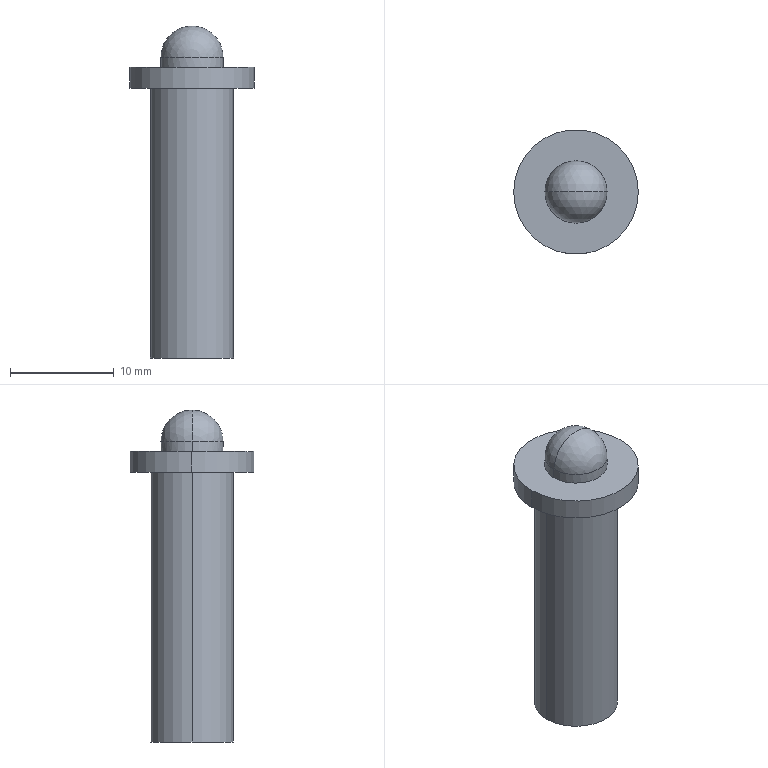Part | STEP file | 2053 Spring mounting seat A | 1 solid | 15 faces | box 12 x 12 x 32 mm | volume 1418 mm3 | cylinder 8 | plane 3 | cone 2 | sphere 2 | commonest cylinder face diameters 4.2 x2 6 x2 8 x2 12 x2
STEP:
#1=CARTESIAN_POINT('',(0.,0.,0.));
#2=DIRECTION('',(0.,0.,1.));
#3=DIRECTION('',(1.,0.,0.));
#4=AXIS2_PLACEMENT_3D('',#1,#2,#3);
#5=CARTESIAN_POINT('',(-2.1,0.,-14.));
#6=VERTEX_POINT('',#5);
#7=CARTESIAN_POINT('',(-2.1,0.,-28.));
#8=VERTEX_POINT('',#7);
#9=CARTESIAN_POINT('',(-2.1,0.,-28.));
#10=DIRECTION('',(0.,0.,-1.));
#11=VECTOR('',#10,1.);
#12=LINE('',#9,#11);
#13=CARTESIAN_POINT('',(0.,0.,-28.));
#14=DIRECTION('',(0.,0.,-1.));
#15=DIRECTION('',(-1.,0.,0.));
#16=AXIS2_PLACEMENT_3D('',#13,#14,#15);
#17=CYLINDRICAL_SURFACE('',#16,2.1);
#18=CARTESIAN_POINT('',(6.283,0.));
#19=DIRECTION('',(0.,1.));
#20=VECTOR('',#19,1.);
#21=LINE('',#18,#20);
#22=(GEOMETRIC_REPRESENTATION_CONTEXT(2)PARAMETRIC_REPRESENTATION_CONTEXT()REPRESENTATION_CONTEXT('',''));
#23=DEFINITIONAL_REPRESENTATION('',(#21),#22);
#24=PCURVE('',#17,#23);
#25=CARTESIAN_POINT('',(0.,0.,-28.));
#26=DIRECTION('',(0.,0.,-1.));
#27=DIRECTION('',(-1.,0.,0.));
#28=AXIS2_PLACEMENT_3D('',#25,#26,#27);
#29=CYLINDRICAL_SURFACE('',#28,2.1);
#30=CARTESIAN_POINT('',(0.,0.));
#31=DIRECTION('',(0.,1.));
#32=VECTOR('',#31,1.);
#33=LINE('',#30,#32);
#34=(GEOMETRIC_REPRESENTATION_CONTEXT(2)PARAMETRIC_REPRESENTATION_CONTEXT()REPRESENTATION_CONTEXT('',''));
#35=DEFINITIONAL_REPRESENTATION('',(#33),#34);
#36=PCURVE('',#29,#35);
#37=SURFACE_CURVE('',#12,(#24,#36),.PCURVE_S1.);
#38=EDGE_CURVE('',#6,#8,#37,.T.);
#39=ORIENTED_EDGE('',*,*,#38,.T.);
#40=CARTESIAN_POINT('',(2.1,0.,-28.));
#41=VERTEX_POINT('',#40);
#42=CARTESIAN_POINT('',(0.,0.,-28.));
#43=DIRECTION('',(0.,0.,-1.));
#44=DIRECTION('',(-1.,0.,0.));
#45=AXIS2_PLACEMENT_3D('',#42,#43,#44);
#46=CIRCLE('',#45,2.1);
#47=CARTESIAN_POINT('',(0.,0.));
#48=DIRECTION('',(1.,0.));
#49=VECTOR('',#48,1.);
#50=LINE('',#47,#49);
#51=(GEOMETRIC_REPRESENTATION_CONTEXT(2)PARAMETRIC_REPRESENTATION_CONTEXT()REPRESENTATION_CONTEXT('',''));
#52=DEFINITIONAL_REPRESENTATION('',(#50),#51);
#53=PCURVE('',#17,#52);
#54=CARTESIAN_POINT('',(0.,0.,-28.));
#55=DIRECTION('',(0.,0.,-1.));
#56=DIRECTION('',(-1.,0.,0.));
#57=AXIS2_PLACEMENT_3D('',#54,#55,#56);
#58=PLANE('',#57);
#59=CARTESIAN_POINT('',(0.,0.));
#60=DIRECTION('',(1.,0.));
#61=AXIS2_PLACEMENT_2D('',#59,#60);
#62=CIRCLE('',#61,2.1);
#63=(GEOMETRIC_REPRESENTATION_CONTEXT(2)PARAMETRIC_REPRESENTATION_CONTEXT()REPRESENTATION_CONTEXT('',''));
#64=DEFINITIONAL_REPRESENTATION('',(#62),#63);
#65=PCURVE('',#58,#64);
#66=SURFACE_CURVE('',#46,(#53,#65),.PCURVE_S1.);
#67=EDGE_CURVE('',#41,#8,#66,.T.);
#68=ORIENTED_EDGE('',*,*,#67,.F.);
#69=CARTESIAN_POINT('',(2.1,0.,-14.));
#70=VERTEX_POINT('',#69);
#71=CARTESIAN_POINT('',(2.1,0.,-28.));
#72=DIRECTION('',(0.,0.,-1.));
#73=VECTOR('',#72,1.);
#74=LINE('',#71,#73);
#75=CARTESIAN_POINT('',(3.142,0.));
#76=DIRECTION('',(0.,1.));
#77=VECTOR('',#76,1.);
#78=LINE('',#75,#77);
#79=(GEOMETRIC_REPRESENTATION_CONTEXT(2)PARAMETRIC_REPRESENTATION_CONTEXT()REPRESENTATION_CONTEXT('',''));
#80=DEFINITIONAL_REPRESENTATION('',(#78),#79);
#81=PCURVE('',#17,#80);
#82=CARTESIAN_POINT('',(3.142,0.));
#83=DIRECTION('',(0.,1.));
#84=VECTOR('',#83,1.);
#85=LINE('',#82,#84);
#86=(GEOMETRIC_REPRESENTATION_CONTEXT(2)PARAMETRIC_REPRESENTATION_CONTEXT()REPRESENTATION_CONTEXT('',''));
#87=DEFINITIONAL_REPRESENTATION('',(#85),#86);
#88=PCURVE('',#29,#87);
#89=SURFACE_CURVE('',#74,(#81,#88),.PCURVE_S1.);
#90=EDGE_CURVE('',#70,#41,#89,.T.);
#91=ORIENTED_EDGE('',*,*,#90,.F.);
#92=CARTESIAN_POINT('',(0.,0.,-14.));
#93=DIRECTION('',(0.,0.,-1.));
#94=DIRECTION('',(-1.,0.,0.));
#95=AXIS2_PLACEMENT_3D('',#92,#93,#94);
#96=CIRCLE('',#95,2.1);
#97=CARTESIAN_POINT('',(0.,-14.));
#98=DIRECTION('',(1.,0.));
#99=VECTOR('',#98,1.);
#100=LINE('',#97,#99);
#101=(GEOMETRIC_REPRESENTATION_CONTEXT(2)PARAMETRIC_REPRESENTATION_CONTEXT()REPRESENTATION_CONTEXT('',''));
#102=DEFINITIONAL_REPRESENTATION('',(#100),#101);
#103=PCURVE('',#17,#102);
#104=CARTESIAN_POINT('',(0.,0.,-14.));
#105=DIRECTION('',(0.,0.,-1.));
#106=DIRECTION('',(-1.,0.,0.));
#107=AXIS2_PLACEMENT_3D('',#104,#105,#106);
#108=CONICAL_SURFACE('',#107,2.1,1.03);
#109=CARTESIAN_POINT('',(0.,0.));
#110=DIRECTION('',(1.,0.));
#111=VECTOR('',#110,1.);
#112=LINE('',#109,#111);
#113=(GEOMETRIC_REPRESENTATION_CONTEXT(2)PARAMETRIC_REPRESENTATION_CONTEXT()REPRESENTATION_CONTEXT('',''));
#114=DEFINITIONAL_REPRESENTATION('',(#112),#113);
#115=PCURVE('',#108,#114);
#116=SURFACE_CURVE('',#96,(#103,#115),.PCURVE_S1.);
#117=EDGE_CURVE('',#70,#6,#116,.T.);
#118=ORIENTED_EDGE('',*,*,#117,.T.);
#119=EDGE_LOOP('',(#39,#68,#91,#118));
#120=FACE_BOUND('',#119,.F.);
#121=ADVANCED_FACE('',(#120),#17,.F.);
#122=ORIENTED_EDGE('',*,*,#117,.F.);
#123=CARTESIAN_POINT('',(0.,0.,-12.738));
#124=VERTEX_POINT('',#123);
#125=CARTESIAN_POINT('',(2.1,0.,-14.));
#126=DIRECTION('',(0.8572,0.,-0.515));
#127=VECTOR('',#126,1.);
#128=LINE('',#125,#127);
#129=CARTESIAN_POINT('',(3.142,0.));
#130=DIRECTION('',(0.,1.));
#131=VECTOR('',#130,1.);
#132=LINE('',#129,#131);
#133=(GEOMETRIC_REPRESENTATION_CONTEXT(2)PARAMETRIC_REPRESENTATION_CONTEXT()REPRESENTATION_CONTEXT('',''));
#134=DEFINITIONAL_REPRESENTATION('',(#132),#133);
#135=PCURVE('',#108,#134);
#136=CARTESIAN_POINT('',(0.,0.,-14.));
#137=DIRECTION('',(0.,0.,-1.));
#138=DIRECTION('',(-1.,0.,0.));
#139=AXIS2_PLACEMENT_3D('',#136,#137,#138);
#140=CONICAL_SURFACE('',#139,2.1,1.03);
#141=CARTESIAN_POINT('',(3.142,0.));
#142=DIRECTION('',(0.,1.));
#143=VECTOR('',#142,1.);
#144=LINE('',#141,#143);
#145=(GEOMETRIC_REPRESENTATION_CONTEXT(2)PARAMETRIC_REPRESENTATION_CONTEXT()REPRESENTATION_CONTEXT('',''));
#146=DEFINITIONAL_REPRESENTATION('',(#144),#145);
#147=PCURVE('',#140,#146);
#148=SURFACE_CURVE('',#128,(#135,#147),.PCURVE_S1.);
#149=EDGE_CURVE('',#124,#70,#148,.T.);
#150=ORIENTED_EDGE('',*,*,#149,.F.);
#151=CARTESIAN_POINT('',(-2.1,0.,-14.));
#152=DIRECTION('',(-0.8572,0.,-0.515));
#153=VECTOR('',#152,1.);
#154=LINE('',#151,#153);
#155=CARTESIAN_POINT('',(6.283,0.));
#156=DIRECTION('',(0.,1.));
#157=VECTOR('',#156,1.);
#158=LINE('',#155,#157);
#159=(GEOMETRIC_REPRESENTATION_CONTEXT(2)PARAMETRIC_REPRESENTATION_CONTEXT()REPRESENTATION_CONTEXT('',''));
#160=DEFINITIONAL_REPRESENTATION('',(#158),#159);
#161=PCURVE('',#108,#160);
#162=CARTESIAN_POINT('',(0.,0.));
#163=DIRECTION('',(0.,1.));
#164=VECTOR('',#163,1.);
#165=LINE('',#162,#164);
#166=(GEOMETRIC_REPRESENTATION_CONTEXT(2)PARAMETRIC_REPRESENTATION_CONTEXT()REPRESENTATION_CONTEXT('',''));
#167=DEFINITIONAL_REPRESENTATION('',(#165),#166);
#168=PCURVE('',#140,#167);
#169=SURFACE_CURVE('',#154,(#161,#168),.PCURVE_S1.);
#170=EDGE_CURVE('',#124,#6,#169,.T.);
#171=ORIENTED_EDGE('',*,*,#170,.T.);
#172=EDGE_LOOP('',(#122,#150,#171));
#173=FACE_BOUND('',#172,.F.);
#174=ADVANCED_FACE('',(#173),#108,.F.);
#175=CARTESIAN_POINT('',(0.,3.,1.));
#176=VERTEX_POINT('',#175);
#177=CARTESIAN_POINT('',(3.,0.,1.));
#178=VERTEX_POINT('',#177);
#179=CARTESIAN_POINT('',(0.,0.,1.));
#180=DIRECTION('',(0.,0.,-1.));
#181=DIRECTION('',(-1.,0.,0.));
#182=AXIS2_PLACEMENT_3D('',#179,#180,#181);
#183=CIRCLE('',#182,3.);
#184=CARTESIAN_POINT('',(0.,0.,1.));
#185=DIRECTION('',(0.,1.,0.));
#186=DIRECTION('',(1.,0.,0.));
#187=AXIS2_PLACEMENT_3D('',#184,#185,#186);
#188=SPHERICAL_SURFACE('',#187,3.);
#189=CARTESIAN_POINT('',(6.283,1.571));
#190=CARTESIAN_POINT('',(6.283,1.547));
#191=CARTESIAN_POINT('',(6.283,1.499));
#192=CARTESIAN_POINT('',(6.283,1.428));
#193=CARTESIAN_POINT('',(6.283,1.357));
#194=CARTESIAN_POINT('',(6.283,1.285));
#195=CARTESIAN_POINT('',(6.283,1.214));
#196=CARTESIAN_POINT('',(6.283,1.142));
#197=CARTESIAN_POINT('',(6.283,1.071));
#198=CARTESIAN_POINT('',(6.283,0.9996));
#199=CARTESIAN_POINT('',(6.283,0.9282));
#200=CARTESIAN_POINT('',(6.283,0.8568));
#201=CARTESIAN_POINT('',(6.283,0.7854));
#202=CARTESIAN_POINT('',(6.283,0.714));
#203=CARTESIAN_POINT('',(6.283,0.6426));
#204=CARTESIAN_POINT('',(6.283,0.5712));
#205=CARTESIAN_POINT('',(6.283,0.4998));
#206=CARTESIAN_POINT('',(6.283,0.4284));
#207=CARTESIAN_POINT('',(6.283,0.357));
#208=CARTESIAN_POINT('',(6.283,0.2856));
#209=CARTESIAN_POINT('',(6.283,0.2142));
#210=CARTESIAN_POINT('',(6.283,0.1428));
#211=CARTESIAN_POINT('',(6.283,0.0714));
#212=CARTESIAN_POINT('',(6.283,0.0238));
#213=CARTESIAN_POINT('',(6.283,0.));
#214=B_SPLINE_CURVE_WITH_KNOTS('',3,(#189,#190,#191,#192,#193,#194,#195,#196,#197,#198,#199,#200,#201,#202,#203,#204,#205,#206,#207,#208,#209,#210,#211,#212,#213),.UNSPECIFIED.,.F.,.F.,(4,1,1,1,1,1,1,1,1,1,1,1,1,1,1,1,1,1,1,1,1,1,4),(1.571,1.642,1.714,1.785,1.856,1.928,1.999,2.071,2.142,2.213,2.285,2.356,2.428,2.499,2.57,2.642,2.713,2.785,2.856,2.927,2.999,3.07,3.142),.QUASI_UNIFORM_KNOTS.);
#215=(GEOMETRIC_REPRESENTATION_CONTEXT(2)PARAMETRIC_REPRESENTATION_CONTEXT()REPRESENTATION_CONTEXT('',''));
#216=DEFINITIONAL_REPRESENTATION('',(#214),#215);
#217=PCURVE('',#188,#216);
#218=CARTESIAN_POINT('',(0.,0.,4.));
#219=DIRECTION('',(0.,0.,-1.));
#220=DIRECTION('',(-1.,0.,0.));
#221=AXIS2_PLACEMENT_3D('',#218,#219,#220);
#222=CYLINDRICAL_SURFACE('',#221,3.);
#223=CARTESIAN_POINT('',(0.,3.));
#224=DIRECTION('',(1.,0.));
#225=VECTOR('',#224,1.);
#226=LINE('',#223,#225);
#227=(GEOMETRIC_REPRESENTATION_CONTEXT(2)PARAMETRIC_REPRESENTATION_CONTEXT()REPRESENTATION_CONTEXT('',''));
#228=DEFINITIONAL_REPRESENTATION('',(#226),#227);
#229=PCURVE('',#222,#228);
#230=SURFACE_CURVE('',#183,(#217,#229),.PCURVE_S1.);
#231=EDGE_CURVE('',#176,#178,#230,.T.);
#232=ORIENTED_EDGE('',*,*,#231,.F.);
#233=CARTESIAN_POINT('',(-3.,0.,1.));
#234=VERTEX_POINT('',#233);
#235=CARTESIAN_POINT('',(0.,0.,1.));
#236=DIRECTION('',(0.,0.,-1.));
#237=DIRECTION('',(-1.,0.,0.));
#238=AXIS2_PLACEMENT_3D('',#235,#236,#237);
#239=CIRCLE('',#238,3.);
#240=CARTESIAN_POINT('',(3.142,0.));
#241=DIRECTION('',(0.,1.));
#242=VECTOR('',#241,1.);
#243=LINE('',#240,#242);
#244=(GEOMETRIC_REPRESENTATION_CONTEXT(2)PARAMETRIC_REPRESENTATION_CONTEXT()REPRESENTATION_CONTEXT('',''));
#245=DEFINITIONAL_REPRESENTATION('',(#243),#244);
#246=PCURVE('',#188,#245);
#247=CARTESIAN_POINT('',(0.,3.));
#248=DIRECTION('',(1.,0.));
#249=VECTOR('',#248,1.);
#250=LINE('',#247,#249);
#251=(GEOMETRIC_REPRESENTATION_CONTEXT(2)PARAMETRIC_REPRESENTATION_CONTEXT()REPRESENTATION_CONTEXT('',''));
#252=DEFINITIONAL_REPRESENTATION('',(#250),#251);
#253=PCURVE('',#222,#252);
#254=SURFACE_CURVE('',#239,(#246,#253),.PCURVE_S1.);
#255=EDGE_CURVE('',#234,#176,#254,.T.);
#256=ORIENTED_EDGE('',*,*,#255,.F.);
#257=CARTESIAN_POINT('',(0.,0.,4.));
#258=VERTEX_POINT('',#257);
#259=CARTESIAN_POINT('',(0.,0.,1.));
#260=DIRECTION('',(0.,1.,0.));
#261=DIRECTION('',(-1.,0.,0.));
#262=AXIS2_PLACEMENT_3D('',#259,#260,#261);
#263=CIRCLE('',#262,3.);
#264=CARTESIAN_POINT('',(3.142,0.));
#265=DIRECTION('',(1.,0.));
#266=VECTOR('',#265,1.);
#267=LINE('',#264,#266);
#268=(GEOMETRIC_REPRESENTATION_CONTEXT(2)PARAMETRIC_REPRESENTATION_CONTEXT()REPRESENTATION_CONTEXT('',''));
#269=DEFINITIONAL_REPRESENTATION('',(#267),#268);
#270=PCURVE('',#188,#269);
#271=CARTESIAN_POINT('',(0.,0.,1.));
#272=DIRECTION('',(0.,1.,0.));
#273=DIRECTION('',(1.,0.,0.));
#274=AXIS2_PLACEMENT_3D('',#271,#272,#273);
#275=SPHERICAL_SURFACE('',#274,3.);
#276=CARTESIAN_POINT('',(3.142,0.));
#277=DIRECTION('',(1.,0.));
#278=VECTOR('',#277,1.);
#279=LINE('',#276,#278);
#280=(GEOMETRIC_REPRESENTATION_CONTEXT(2)PARAMETRIC_REPRESENTATION_CONTEXT()REPRESENTATION_CONTEXT('',''));
#281=DEFINITIONAL_REPRESENTATION('',(#279),#280);
#282=PCURVE('',#275,#281);
#283=SURFACE_CURVE('',#263,(#270,#282),.PCURVE_S1.);
#284=EDGE_CURVE('',#234,#258,#283,.T.);
#285=ORIENTED_EDGE('',*,*,#284,.T.);
#286=CARTESIAN_POINT('',(0.,0.,1.));
#287=DIRECTION('',(0.,-1.,0.));
#288=DIRECTION('',(0.,0.,-1.));
#289=AXIS2_PLACEMENT_3D('',#286,#287,#288);
#290=CIRCLE('',#289,3.);
#291=CARTESIAN_POINT('',(6.283,0.));
#292=CARTESIAN_POINT('',(6.259,0.));
#293=CARTESIAN_POINT('',(6.212,0.));
#294=CARTESIAN_POINT('',(6.14,0.));
#295=CARTESIAN_POINT('',(6.069,0.));
#296=CARTESIAN_POINT('',(5.998,0.));
#297=CARTESIAN_POINT('',(5.926,0.));
#298=CARTESIAN_POINT('',(5.855,0.));
#299=CARTESIAN_POINT('',(5.783,0.));
#300=CARTESIAN_POINT('',(5.712,0.));
#301=CARTESIAN_POINT('',(5.641,0.));
#302=CARTESIAN_POINT('',(5.569,0.));
#303=CARTESIAN_POINT('',(5.498,0.));
#304=CARTESIAN_POINT('',(5.426,0.));
#305=CARTESIAN_POINT('',(5.355,0.));
#306=CARTESIAN_POINT('',(5.284,0.));
#307=CARTESIAN_POINT('',(5.212,0.));
#308=CARTESIAN_POINT('',(5.141,0.));
#309=CARTESIAN_POINT('',(5.069,0.));
#310=CARTESIAN_POINT('',(4.998,0.));
#311=CARTESIAN_POINT('',(4.927,0.));
#312=CARTESIAN_POINT('',(4.855,0.));
#313=CARTESIAN_POINT('',(4.784,0.));
#314=CARTESIAN_POINT('',(4.736,0.));
#315=CARTESIAN_POINT('',(4.712,0.));
#316=B_SPLINE_CURVE_WITH_KNOTS('',3,(#291,#292,#293,#294,#295,#296,#297,#298,#299,#300,#301,#302,#303,#304,#305,#306,#307,#308,#309,#310,#311,#312,#313,#314,#315),.UNSPECIFIED.,.F.,.F.,(4,1,1,1,1,1,1,1,1,1,1,1,1,1,1,1,1,1,1,1,1,1,4),(1.571,1.642,1.714,1.785,1.856,1.928,1.999,2.071,2.142,2.213,2.285,2.356,2.428,2.499,2.57,2.642,2.713,2.785,2.856,2.927,2.999,3.07,3.142),.QUASI_UNIFORM_KNOTS.);
#317=(GEOMETRIC_REPRESENTATION_CONTEXT(2)PARAMETRIC_REPRESENTATION_CONTEXT()REPRESENTATION_CONTEXT('',''));
#318=DEFINITIONAL_REPRESENTATION('',(#316),#317);
#319=PCURVE('',#188,#318);
#320=CARTESIAN_POINT('',(6.283,0.));
#321=CARTESIAN_POINT('',(6.259,0.));
#322=CARTESIAN_POINT('',(6.212,0.));
#323=CARTESIAN_POINT('',(6.14,0.));
#324=CARTESIAN_POINT('',(6.069,0.));
#325=CARTESIAN_POINT('',(5.998,0.));
#326=CARTESIAN_POINT('',(5.926,0.));
#327=CARTESIAN_POINT('',(5.855,0.));
#328=CARTESIAN_POINT('',(5.783,0.));
#329=CARTESIAN_POINT('',(5.712,0.));
#330=CARTESIAN_POINT('',(5.641,0.));
#331=CARTESIAN_POINT('',(5.569,0.));
#332=CARTESIAN_POINT('',(5.498,0.));
#333=CARTESIAN_POINT('',(5.426,0.));
#334=CARTESIAN_POINT('',(5.355,0.));
#335=CARTESIAN_POINT('',(5.284,0.));
#336=CARTESIAN_POINT('',(5.212,0.));
#337=CARTESIAN_POINT('',(5.141,0.));
#338=CARTESIAN_POINT('',(5.069,0.));
#339=CARTESIAN_POINT('',(4.998,0.));
#340=CARTESIAN_POINT('',(4.927,0.));
#341=CARTESIAN_POINT('',(4.855,0.));
#342=CARTESIAN_POINT('',(4.784,0.));
#343=CARTESIAN_POINT('',(4.736,0.));
#344=CARTESIAN_POINT('',(4.712,0.));
#345=B_SPLINE_CURVE_WITH_KNOTS('',3,(#320,#321,#322,#323,#324,#325,#326,#327,#328,#329,#330,#331,#332,#333,#334,#335,#336,#337,#338,#339,#340,#341,#342,#343,#344),.UNSPECIFIED.,.F.,.F.,(4,1,1,1,1,1,1,1,1,1,1,1,1,1,1,1,1,1,1,1,1,1,4),(1.571,1.642,1.714,1.785,1.856,1.928,1.999,2.071,2.142,2.213,2.285,2.356,2.428,2.499,2.57,2.642,2.713,2.785,2.856,2.927,2.999,3.07,3.142),.QUASI_UNIFORM_KNOTS.);
#346=(GEOMETRIC_REPRESENTATION_CONTEXT(2)PARAMETRIC_REPRESENTATION_CONTEXT()REPRESENTATION_CONTEXT('',''));
#347=DEFINITIONAL_REPRESENTATION('',(#345),#346);
#348=PCURVE('',#275,#347);
#349=SURFACE_CURVE('',#290,(#319,#348),.PCURVE_S1.);
#350=EDGE_CURVE('',#178,#258,#349,.T.);
#351=ORIENTED_EDGE('',*,*,#350,.F.);
#352=EDGE_LOOP('',(#232,#256,#285,#351));
#353=FACE_BOUND('',#352,.T.);
#354=ADVANCED_FACE('',(#353),#188,.T.);
#355=CARTESIAN_POINT('',(-4.,0.,-28.));
#356=VERTEX_POINT('',#355);
#357=CARTESIAN_POINT('',(4.,0.,-28.));
#358=VERTEX_POINT('',#357);
#359=CARTESIAN_POINT('',(0.,0.,-28.));
#360=DIRECTION('',(0.,0.,-1.));
#361=DIRECTION('',(-1.,0.,0.));
#362=AXIS2_PLACEMENT_3D('',#359,#360,#361);
#363=CIRCLE('',#362,4.);
#364=CARTESIAN_POINT('',(0.,0.,-28.));
#365=DIRECTION('',(0.,0.,1.));
#366=DIRECTION('',(1.,0.,0.));
#367=AXIS2_PLACEMENT_3D('',#364,#365,#366);
#368=CYLINDRICAL_SURFACE('',#367,4.);
#369=CARTESIAN_POINT('',(3.142,0.));
#370=DIRECTION('',(-1.,0.));
#371=VECTOR('',#370,1.);
#372=LINE('',#369,#371);
#373=(GEOMETRIC_REPRESENTATION_CONTEXT(2)PARAMETRIC_REPRESENTATION_CONTEXT()REPRESENTATION_CONTEXT('',''));
#374=DEFINITIONAL_REPRESENTATION('',(#372),#373);
#375=PCURVE('',#368,#374);
#376=CARTESIAN_POINT('',(0.,0.));
#377=DIRECTION('',(1.,0.));
#378=AXIS2_PLACEMENT_2D('',#376,#377);
#379=CIRCLE('',#378,4.);
#380=(GEOMETRIC_REPRESENTATION_CONTEXT(2)PARAMETRIC_REPRESENTATION_CONTEXT()REPRESENTATION_CONTEXT('',''));
#381=DEFINITIONAL_REPRESENTATION('',(#379),#380);
#382=PCURVE('',#58,#381);
#383=SURFACE_CURVE('',#363,(#375,#382),.PCURVE_S1.);
#384=EDGE_CURVE('',#356,#358,#383,.T.);
#385=ORIENTED_EDGE('',*,*,#384,.F.);
#386=CARTESIAN_POINT('',(-4.,0.,-2.));
#387=VERTEX_POINT('',#386);
#388=CARTESIAN_POINT('',(-4.,0.,-28.));
#389=DIRECTION('',(0.,0.,1.));
#390=VECTOR('',#389,1.);
#391=LINE('',#388,#390);
#392=CARTESIAN_POINT('',(3.142,0.));
#393=DIRECTION('',(0.,1.));
#394=VECTOR('',#393,1.);
#395=LINE('',#392,#394);
#396=(GEOMETRIC_REPRESENTATION_CONTEXT(2)PARAMETRIC_REPRESENTATION_CONTEXT()REPRESENTATION_CONTEXT('',''));
#397=DEFINITIONAL_REPRESENTATION('',(#395),#396);
#398=PCURVE('',#368,#397);
#399=CARTESIAN_POINT('',(0.,0.,-28.));
#400=DIRECTION('',(0.,0.,1.));
#401=DIRECTION('',(1.,0.,0.));
#402=AXIS2_PLACEMENT_3D('',#399,#400,#401);
#403=CYLINDRICAL_SURFACE('',#402,4.);
#404=CARTESIAN_POINT('',(3.142,0.));
#405=DIRECTION('',(0.,1.));
#406=VECTOR('',#405,1.);
#407=LINE('',#404,#406);
#408=(GEOMETRIC_REPRESENTATION_CONTEXT(2)PARAMETRIC_REPRESENTATION_CONTEXT()REPRESENTATION_CONTEXT('',''));
#409=DEFINITIONAL_REPRESENTATION('',(#407),#408);
#410=PCURVE('',#403,#409);
#411=SURFACE_CURVE('',#391,(#398,#410),.PCURVE_S1.);
#412=EDGE_CURVE('',#356,#387,#411,.T.);
#413=ORIENTED_EDGE('',*,*,#412,.T.);
#414=CARTESIAN_POINT('',(4.,0.,-2.));
#415=VERTEX_POINT('',#414);
#416=CARTESIAN_POINT('',(0.,0.,-2.));
#417=DIRECTION('',(0.,0.,-1.));
#418=DIRECTION('',(-1.,0.,0.));
#419=AXIS2_PLACEMENT_3D('',#416,#417,#418);
#420=CIRCLE('',#419,4.);
#421=CARTESIAN_POINT('',(3.142,26.));
#422=DIRECTION('',(-1.,0.));
#423=VECTOR('',#422,1.);
#424=LINE('',#421,#423);
#425=(GEOMETRIC_REPRESENTATION_CONTEXT(2)PARAMETRIC_REPRESENTATION_CONTEXT()REPRESENTATION_CONTEXT('',''));
#426=DEFINITIONAL_REPRESENTATION('',(#424),#425);
#427=PCURVE('',#368,#426);
#428=CARTESIAN_POINT('',(0.,0.,-2.));
#429=DIRECTION('',(0.,0.,-1.));
#430=DIRECTION('',(-1.,0.,0.));
#431=AXIS2_PLACEMENT_3D('',#428,#429,#430);
#432=PLANE('',#431);
#433=CARTESIAN_POINT('',(0.,0.));
#434=DIRECTION('',(1.,0.));
#435=AXIS2_PLACEMENT_2D('',#433,#434);
#436=CIRCLE('',#435,4.);
#437=(GEOMETRIC_REPRESENTATION_CONTEXT(2)PARAMETRIC_REPRESENTATION_CONTEXT()REPRESENTATION_CONTEXT('',''));
#438=DEFINITIONAL_REPRESENTATION('',(#436),#437);
#439=PCURVE('',#432,#438);
#440=SURFACE_CURVE('',#420,(#427,#439),.PCURVE_S1.);
#441=EDGE_CURVE('',#387,#415,#440,.T.);
#442=ORIENTED_EDGE('',*,*,#441,.T.);
#443=CARTESIAN_POINT('',(4.,0.,-28.));
#444=DIRECTION('',(0.,0.,1.));
#445=VECTOR('',#444,1.);
#446=LINE('',#443,#445);
#447=CARTESIAN_POINT('',(0.,0.));
#448=DIRECTION('',(0.,1.));
#449=VECTOR('',#448,1.);
#450=LINE('',#447,#449);
#451=(GEOMETRIC_REPRESENTATION_CONTEXT(2)PARAMETRIC_REPRESENTATION_CONTEXT()REPRESENTATION_CONTEXT('',''));
#452=DEFINITIONAL_REPRESENTATION('',(#450),#451);
#453=PCURVE('',#368,#452);
#454=CARTESIAN_POINT('',(6.283,0.));
#455=DIRECTION('',(0.,1.));
#456=VECTOR('',#455,1.);
#457=LINE('',#454,#456);
#458=(GEOMETRIC_REPRESENTATION_CONTEXT(2)PARAMETRIC_REPRESENTATION_CONTEXT()REPRESENTATION_CONTEXT('',''));
#459=DEFINITIONAL_REPRESENTATION('',(#457),#458);
#460=PCURVE('',#403,#459);
#461=SURFACE_CURVE('',#446,(#453,#460),.PCURVE_S1.);
#462=EDGE_CURVE('',#358,#415,#461,.T.);
#463=ORIENTED_EDGE('',*,*,#462,.F.);
#464=EDGE_LOOP('',(#385,#413,#442,#463));
#465=FACE_BOUND('',#464,.T.);
#466=ADVANCED_FACE('',(#465),#368,.T.);
#467=CARTESIAN_POINT('',(-6.,0.,-2.));
#468=VERTEX_POINT('',#467);
#469=CARTESIAN_POINT('',(6.,0.,-2.));
#470=VERTEX_POINT('',#469);
#471=CARTESIAN_POINT('',(0.,0.,-2.));
#472=DIRECTION('',(0.,0.,-1.));
#473=DIRECTION('',(-1.,0.,0.));
#474=AXIS2_PLACEMENT_3D('',#471,#472,#473);
#475=CIRCLE('',#474,6.);
#476=CARTESIAN_POINT('',(0.,0.,-2.));
#477=DIRECTION('',(0.,0.,1.));
#478=DIRECTION('',(1.,0.,0.));
#479=AXIS2_PLACEMENT_3D('',#476,#477,#478);
#480=CYLINDRICAL_SURFACE('',#479,6.);
#481=CARTESIAN_POINT('',(3.142,0.));
#482=DIRECTION('',(-1.,0.));
#483=VECTOR('',#482,1.);
#484=LINE('',#481,#483);
#485=(GEOMETRIC_REPRESENTATION_CONTEXT(2)PARAMETRIC_REPRESENTATION_CONTEXT()REPRESENTATION_CONTEXT('',''));
#486=DEFINITIONAL_REPRESENTATION('',(#484),#485);
#487=PCURVE('',#480,#486);
#488=CARTESIAN_POINT('',(0.,0.));
#489=DIRECTION('',(1.,0.));
#490=AXIS2_PLACEMENT_2D('',#488,#489);
#491=CIRCLE('',#490,6.);
#492=(GEOMETRIC_REPRESENTATION_CONTEXT(2)PARAMETRIC_REPRESENTATION_CONTEXT()REPRESENTATION_CONTEXT('',''));
#493=DEFINITIONAL_REPRESENTATION('',(#491),#492);
#494=PCURVE('',#432,#493);
#495=SURFACE_CURVE('',#475,(#487,#494),.PCURVE_S1.);
#496=EDGE_CURVE('',#468,#470,#495,.T.);
#497=ORIENTED_EDGE('',*,*,#496,.F.);
#498=CARTESIAN_POINT('',(-6.,0.,0.));
#499=VERTEX_POINT('',#498);
#500=CARTESIAN_POINT('',(-6.,0.,-2.));
#501=DIRECTION('',(0.,0.,1.));
#502=VECTOR('',#501,1.);
#503=LINE('',#500,#502);
#504=CARTESIAN_POINT('',(3.142,0.));
#505=DIRECTION('',(0.,1.));
#506=VECTOR('',#505,1.);
#507=LINE('',#504,#506);
#508=(GEOMETRIC_REPRESENTATION_CONTEXT(2)PARAMETRIC_REPRESENTATION_CONTEXT()REPRESENTATION_CONTEXT('',''));
#509=DEFINITIONAL_REPRESENTATION('',(#507),#508);
#510=PCURVE('',#480,#509);
#511=CARTESIAN_POINT('',(0.,0.,-2.));
#512=DIRECTION('',(0.,0.,1.));
#513=DIRECTION('',(1.,0.,0.));
#514=AXIS2_PLACEMENT_3D('',#511,#512,#513);
#515=CYLINDRICAL_SURFACE('',#514,6.);
#516=CARTESIAN_POINT('',(3.142,0.));
#517=DIRECTION('',(0.,1.));
#518=VECTOR('',#517,1.);
#519=LINE('',#516,#518);
#520=(GEOMETRIC_REPRESENTATION_CONTEXT(2)PARAMETRIC_REPRESENTATION_CONTEXT()REPRESENTATION_CONTEXT('',''));
#521=DEFINITIONAL_REPRESENTATION('',(#519),#520);
#522=PCURVE('',#515,#521);
#523=SURFACE_CURVE('',#503,(#510,#522),.PCURVE_S1.);
#524=EDGE_CURVE('',#468,#499,#523,.T.);
#525=ORIENTED_EDGE('',*,*,#524,.T.);
#526=CARTESIAN_POINT('',(6.,0.,0.));
#527=VERTEX_POINT('',#526);
#528=CARTESIAN_POINT('',(0.,0.,0.));
#529=DIRECTION('',(0.,0.,-1.));
#530=DIRECTION('',(-1.,0.,0.));
#531=AXIS2_PLACEMENT_3D('',#528,#529,#530);
#532=CIRCLE('',#531,6.);
#533=CARTESIAN_POINT('',(3.142,2.));
#534=DIRECTION('',(-1.,0.));
#535=VECTOR('',#534,1.);
#536=LINE('',#533,#535);
#537=(GEOMETRIC_REPRESENTATION_CONTEXT(2)PARAMETRIC_REPRESENTATION_CONTEXT()REPRESENTATION_CONTEXT('',''));
#538=DEFINITIONAL_REPRESENTATION('',(#536),#537);
#539=PCURVE('',#480,#538);
#540=CARTESIAN_POINT('',(0.,0.,0.));
#541=DIRECTION('',(0.,0.,-1.));
#542=DIRECTION('',(-1.,0.,0.));
#543=AXIS2_PLACEMENT_3D('',#540,#541,#542);
#544=PLANE('',#543);
#545=CARTESIAN_POINT('',(0.,0.));
#546=DIRECTION('',(1.,0.));
#547=AXIS2_PLACEMENT_2D('',#545,#546);
#548=CIRCLE('',#547,6.);
#549=(GEOMETRIC_REPRESENTATION_CONTEXT(2)PARAMETRIC_REPRESENTATION_CONTEXT()REPRESENTATION_CONTEXT('',''));
#550=DEFINITIONAL_REPRESENTATION('',(#548),#549);
#551=PCURVE('',#544,#550);
#552=SURFACE_CURVE('',#532,(#539,#551),.PCURVE_S1.);
#553=EDGE_CURVE('',#499,#527,#552,.T.);
#554=ORIENTED_EDGE('',*,*,#553,.T.);
#555=CARTESIAN_POINT('',(6.,0.,-2.));
#556=DIRECTION('',(0.,0.,1.));
#557=VECTOR('',#556,1.);
#558=LINE('',#555,#557);
#559=CARTESIAN_POINT('',(0.,0.));
#560=DIRECTION('',(0.,1.));
#561=VECTOR('',#560,1.);
#562=LINE('',#559,#561);
#563=(GEOMETRIC_REPRESENTATION_CONTEXT(2)PARAMETRIC_REPRESENTATION_CONTEXT()REPRESENTATION_CONTEXT('',''));
#564=DEFINITIONAL_REPRESENTATION('',(#562),#563);
#565=PCURVE('',#480,#564);
#566=CARTESIAN_POINT('',(6.283,0.));
#567=DIRECTION('',(0.,1.));
#568=VECTOR('',#567,1.);
#569=LINE('',#566,#568);
#570=(GEOMETRIC_REPRESENTATION_CONTEXT(2)PARAMETRIC_REPRESENTATION_CONTEXT()REPRESENTATION_CONTEXT('',''));
#571=DEFINITIONAL_REPRESENTATION('',(#569),#570);
#572=PCURVE('',#515,#571);
#573=SURFACE_CURVE('',#558,(#565,#572),.PCURVE_S1.);
#574=EDGE_CURVE('',#470,#527,#573,.T.);
#575=ORIENTED_EDGE('',*,*,#574,.F.);
#576=EDGE_LOOP('',(#497,#525,#554,#575));
#577=FACE_BOUND('',#576,.T.);
#578=ADVANCED_FACE('',(#577),#480,.T.);
#579=ORIENTED_EDGE('',*,*,#231,.T.);
#580=CARTESIAN_POINT('',(3.,0.,0.));
#581=VERTEX_POINT('',#580);
#582=CARTESIAN_POINT('',(3.,0.,4.));
#583=DIRECTION('',(0.,0.,-1.));
#584=VECTOR('',#583,1.);
#585=LINE('',#582,#584);
#586=CARTESIAN_POINT('',(3.142,0.));
#587=DIRECTION('',(0.,1.));
#588=VECTOR('',#587,1.);
#589=LINE('',#586,#588);
#590=(GEOMETRIC_REPRESENTATION_CONTEXT(2)PARAMETRIC_REPRESENTATION_CONTEXT()REPRESENTATION_CONTEXT('',''));
#591=DEFINITIONAL_REPRESENTATION('',(#589),#590);
#592=PCURVE('',#222,#591);
#593=CARTESIAN_POINT('',(0.,0.,4.));
#594=DIRECTION('',(0.,0.,-1.));
#595=DIRECTION('',(-1.,0.,0.));
#596=AXIS2_PLACEMENT_3D('',#593,#594,#595);
#597=CYLINDRICAL_SURFACE('',#596,3.);
#598=CARTESIAN_POINT('',(3.142,0.));
#599=DIRECTION('',(0.,1.));
#600=VECTOR('',#599,1.);
#601=LINE('',#598,#600);
#602=(GEOMETRIC_REPRESENTATION_CONTEXT(2)PARAMETRIC_REPRESENTATION_CONTEXT()REPRESENTATION_CONTEXT('',''));
#603=DEFINITIONAL_REPRESENTATION('',(#601),#602);
#604=PCURVE('',#597,#603);
#605=SURFACE_CURVE('',#585,(#592,#604),.PCURVE_S1.);
#606=EDGE_CURVE('',#178,#581,#605,.T.);
#607=ORIENTED_EDGE('',*,*,#606,.T.);
#608=CARTESIAN_POINT('',(-3.,0.,0.));
#609=VERTEX_POINT('',#608);
#610=CARTESIAN_POINT('',(0.,0.,0.));
#611=DIRECTION('',(0.,0.,-1.));
#612=DIRECTION('',(-1.,0.,0.));
#613=AXIS2_PLACEMENT_3D('',#610,#611,#612);
#614=CIRCLE('',#613,3.);
#615=CARTESIAN_POINT('',(0.,4.));
#616=DIRECTION('',(1.,0.));
#617=VECTOR('',#616,1.);
#618=LINE('',#615,#617);
#619=(GEOMETRIC_REPRESENTATION_CONTEXT(2)PARAMETRIC_REPRESENTATION_CONTEXT()REPRESENTATION_CONTEXT('',''));
#620=DEFINITIONAL_REPRESENTATION('',(#618),#619);
#621=PCURVE('',#222,#620);
#622=CARTESIAN_POINT('',(0.,0.));
#623=DIRECTION('',(1.,0.));
#624=AXIS2_PLACEMENT_2D('',#622,#623);
#625=CIRCLE('',#624,3.);
#626=(GEOMETRIC_REPRESENTATION_CONTEXT(2)PARAMETRIC_REPRESENTATION_CONTEXT()REPRESENTATION_CONTEXT('',''));
#627=DEFINITIONAL_REPRESENTATION('',(#625),#626);
#628=PCURVE('',#544,#627);
#629=SURFACE_CURVE('',#614,(#621,#628),.PCURVE_S1.);
#630=EDGE_CURVE('',#609,#581,#629,.T.);
#631=ORIENTED_EDGE('',*,*,#630,.F.);
#632=CARTESIAN_POINT('',(-3.,0.,4.));
#633=DIRECTION('',(0.,0.,-1.));
#634=VECTOR('',#633,1.);
#635=LINE('',#632,#634);
#636=CARTESIAN_POINT('',(0.,0.));
#637=DIRECTION('',(0.,1.));
#638=VECTOR('',#637,1.);
#639=LINE('',#636,#638);
#640=(GEOMETRIC_REPRESENTATION_CONTEXT(2)PARAMETRIC_REPRESENTATION_CONTEXT()REPRESENTATION_CONTEXT('',''));
#641=DEFINITIONAL_REPRESENTATION('',(#639),#640);
#642=PCURVE('',#222,#641);
#643=CARTESIAN_POINT('',(6.283,0.));
#644=DIRECTION('',(0.,1.));
#645=VECTOR('',#644,1.);
#646=LINE('',#643,#645);
#647=(GEOMETRIC_REPRESENTATION_CONTEXT(2)PARAMETRIC_REPRESENTATION_CONTEXT()REPRESENTATION_CONTEXT('',''));
#648=DEFINITIONAL_REPRESENTATION('',(#646),#647);
#649=PCURVE('',#597,#648);
#650=SURFACE_CURVE('',#635,(#642,#649),.PCURVE_S1.);
#651=EDGE_CURVE('',#234,#609,#650,.T.);
#652=ORIENTED_EDGE('',*,*,#651,.F.);
#653=ORIENTED_EDGE('',*,*,#255,.T.);
#654=EDGE_LOOP('',(#579,#607,#631,#652,#653));
#655=FACE_BOUND('',#654,.T.);
#656=ADVANCED_FACE('',(#655),#222,.T.);
#657=CARTESIAN_POINT('',(0.,0.,-2.));
#658=DIRECTION('',(0.,0.,-1.));
#659=DIRECTION('',(-1.,0.,0.));
#660=AXIS2_PLACEMENT_3D('',#657,#658,#659);
#661=CIRCLE('',#660,6.);
#662=CARTESIAN_POINT('',(0.,0.));
#663=DIRECTION('',(1.,0.));
#664=AXIS2_PLACEMENT_2D('',#662,#663);
#665=CIRCLE('',#664,6.);
#666=(GEOMETRIC_REPRESENTATION_CONTEXT(2)PARAMETRIC_REPRESENTATION_CONTEXT()REPRESENTATION_CONTEXT('',''));
#667=DEFINITIONAL_REPRESENTATION('',(#665),#666);
#668=PCURVE('',#432,#667);
#669=CARTESIAN_POINT('',(9.425,0.));
#670=DIRECTION('',(-1.,0.));
#671=VECTOR('',#670,1.);
#672=LINE('',#669,#671);
#673=(GEOMETRIC_REPRESENTATION_CONTEXT(2)PARAMETRIC_REPRESENTATION_CONTEXT()REPRESENTATION_CONTEXT('',''));
#674=DEFINITIONAL_REPRESENTATION('',(#672),#673);
#675=PCURVE('',#515,#674);
#676=SURFACE_CURVE('',#661,(#668,#675),.PCURVE_S1.);
#677=EDGE_CURVE('',#470,#468,#676,.T.);
#678=ORIENTED_EDGE('',*,*,#677,.T.);
#679=ORIENTED_EDGE('',*,*,#496,.T.);
#680=EDGE_LOOP('',(#678,#679));
#681=FACE_BOUND('',#680,.T.);
#682=CARTESIAN_POINT('',(0.,0.,-2.));
#683=DIRECTION('',(0.,0.,-1.));
#684=DIRECTION('',(-1.,0.,0.));
#685=AXIS2_PLACEMENT_3D('',#682,#683,#684);
#686=CIRCLE('',#685,4.);
#687=CARTESIAN_POINT('',(0.,0.));
#688=DIRECTION('',(1.,0.));
#689=AXIS2_PLACEMENT_2D('',#687,#688);
#690=CIRCLE('',#689,4.);
#691=(GEOMETRIC_REPRESENTATION_CONTEXT(2)PARAMETRIC_REPRESENTATION_CONTEXT()REPRESENTATION_CONTEXT('',''));
#692=DEFINITIONAL_REPRESENTATION('',(#690),#691);
#693=PCURVE('',#432,#692);
#694=CARTESIAN_POINT('',(9.425,26.));
#695=DIRECTION('',(-1.,0.));
#696=VECTOR('',#695,1.);
#697=LINE('',#694,#696);
#698=(GEOMETRIC_REPRESENTATION_CONTEXT(2)PARAMETRIC_REPRESENTATION_CONTEXT()REPRESENTATION_CONTEXT('',''));
#699=DEFINITIONAL_REPRESENTATION('',(#697),#698);
#700=PCURVE('',#403,#699);
#701=SURFACE_CURVE('',#686,(#693,#700),.PCURVE_S1.);
#702=EDGE_CURVE('',#415,#387,#701,.T.);
#703=ORIENTED_EDGE('',*,*,#702,.F.);
#704=ORIENTED_EDGE('',*,*,#441,.F.);
#705=EDGE_LOOP('',(#703,#704));
#706=FACE_BOUND('',#705,.T.);
#707=ADVANCED_FACE('',(#681,#706),#432,.T.);
#708=ORIENTED_EDGE('',*,*,#606,.F.);
#709=CARTESIAN_POINT('',(0.,-3.,1.));
#710=VERTEX_POINT('',#709);
#711=CARTESIAN_POINT('',(0.,0.,1.));
#712=DIRECTION('',(0.,0.,-1.));
#713=DIRECTION('',(-1.,0.,0.));
#714=AXIS2_PLACEMENT_3D('',#711,#712,#713);
#715=CIRCLE('',#714,3.);
#716=CARTESIAN_POINT('',(0.,3.));
#717=DIRECTION('',(1.,0.));
#718=VECTOR('',#717,1.);
#719=LINE('',#716,#718);
#720=(GEOMETRIC_REPRESENTATION_CONTEXT(2)PARAMETRIC_REPRESENTATION_CONTEXT()REPRESENTATION_CONTEXT('',''));
#721=DEFINITIONAL_REPRESENTATION('',(#719),#720);
#722=PCURVE('',#597,#721);
#723=CARTESIAN_POINT('',(6.283,3.142));
#724=DIRECTION('',(0.,-1.));
#725=VECTOR('',#724,1.);
#726=LINE('',#723,#725);
#727=(GEOMETRIC_REPRESENTATION_CONTEXT(2)PARAMETRIC_REPRESENTATION_CONTEXT()REPRESENTATION_CONTEXT('',''));
#728=DEFINITIONAL_REPRESENTATION('',(#726),#727);
#729=PCURVE('',#275,#728);
#730=SURFACE_CURVE('',#715,(#722,#729),.PCURVE_S1.);
#731=EDGE_CURVE('',#178,#710,#730,.T.);
#732=ORIENTED_EDGE('',*,*,#731,.T.);
#733=CARTESIAN_POINT('',(0.,0.,1.));
#734=DIRECTION('',(0.,0.,-1.));
#735=DIRECTION('',(-1.,0.,0.));
#736=AXIS2_PLACEMENT_3D('',#733,#734,#735);
#737=CIRCLE('',#736,3.);
#738=CARTESIAN_POINT('',(0.,3.));
#739=DIRECTION('',(1.,0.));
#740=VECTOR('',#739,1.);
#741=LINE('',#738,#740);
#742=(GEOMETRIC_REPRESENTATION_CONTEXT(2)PARAMETRIC_REPRESENTATION_CONTEXT()REPRESENTATION_CONTEXT('',''));
#743=DEFINITIONAL_REPRESENTATION('',(#741),#742);
#744=PCURVE('',#597,#743);
#745=CARTESIAN_POINT('',(3.142,-1.571));
#746=CARTESIAN_POINT('',(3.142,-1.547));
#747=CARTESIAN_POINT('',(3.142,-1.499));
#748=CARTESIAN_POINT('',(3.142,-1.428));
#749=CARTESIAN_POINT('',(3.142,-1.357));
#750=CARTESIAN_POINT('',(3.142,-1.285));
#751=CARTESIAN_POINT('',(3.142,-1.214));
#752=CARTESIAN_POINT('',(3.142,-1.142));
#753=CARTESIAN_POINT('',(3.142,-1.071));
#754=CARTESIAN_POINT('',(3.142,-0.9996));
#755=CARTESIAN_POINT('',(3.142,-0.9282));
#756=CARTESIAN_POINT('',(3.142,-0.8568));
#757=CARTESIAN_POINT('',(3.142,-0.7854));
#758=CARTESIAN_POINT('',(3.142,-0.714));
#759=CARTESIAN_POINT('',(3.142,-0.6426));
#760=CARTESIAN_POINT('',(3.142,-0.5712));
#761=CARTESIAN_POINT('',(3.142,-0.4998));
#762=CARTESIAN_POINT('',(3.142,-0.4284));
#763=CARTESIAN_POINT('',(3.142,-0.357));
#764=CARTESIAN_POINT('',(3.142,-0.2856));
#765=CARTESIAN_POINT('',(3.142,-0.2142));
#766=CARTESIAN_POINT('',(3.142,-0.1428));
#767=CARTESIAN_POINT('',(3.142,-0.0714));
#768=CARTESIAN_POINT('',(3.142,-0.0238));
#769=CARTESIAN_POINT('',(3.142,0.));
#770=B_SPLINE_CURVE_WITH_KNOTS('',3,(#745,#746,#747,#748,#749,#750,#751,#752,#753,#754,#755,#756,#757,#758,#759,#760,#761,#762,#763,#764,#765,#766,#767,#768,#769),.UNSPECIFIED.,.F.,.F.,(4,1,1,1,1,1,1,1,1,1,1,1,1,1,1,1,1,1,1,1,1,1,4),(4.712,4.784,4.855,4.927,4.998,5.069,5.141,5.212,5.284,5.355,5.426,5.498,5.569,5.641,5.712,5.783,5.855,5.926,5.998,6.069,6.14,6.212,6.283),.QUASI_UNIFORM_KNOTS.);
#771=(GEOMETRIC_REPRESENTATION_CONTEXT(2)PARAMETRIC_REPRESENTATION_CONTEXT()REPRESENTATION_CONTEXT('',''));
#772=DEFINITIONAL_REPRESENTATION('',(#770),#771);
#773=PCURVE('',#275,#772);
#774=SURFACE_CURVE('',#737,(#744,#773),.PCURVE_S1.);
#775=EDGE_CURVE('',#710,#234,#774,.T.);
#776=ORIENTED_EDGE('',*,*,#775,.T.);
#777=ORIENTED_EDGE('',*,*,#651,.T.);
#778=CARTESIAN_POINT('',(0.,0.,0.));
#779=DIRECTION('',(0.,0.,-1.));
#780=DIRECTION('',(-1.,0.,0.));
#781=AXIS2_PLACEMENT_3D('',#778,#779,#780);
#782=CIRCLE('',#781,3.);
#783=CARTESIAN_POINT('',(0.,4.));
#784=DIRECTION('',(1.,0.));
#785=VECTOR('',#784,1.);
#786=LINE('',#783,#785);
#787=(GEOMETRIC_REPRESENTATION_CONTEXT(2)PARAMETRIC_REPRESENTATION_CONTEXT()REPRESENTATION_CONTEXT('',''));
#788=DEFINITIONAL_REPRESENTATION('',(#786),#787);
#789=PCURVE('',#597,#788);
#790=CARTESIAN_POINT('',(0.,0.));
#791=DIRECTION('',(1.,0.));
#792=AXIS2_PLACEMENT_2D('',#790,#791);
#793=CIRCLE('',#792,3.);
#794=(GEOMETRIC_REPRESENTATION_CONTEXT(2)PARAMETRIC_REPRESENTATION_CONTEXT()REPRESENTATION_CONTEXT('',''));
#795=DEFINITIONAL_REPRESENTATION('',(#793),#794);
#796=PCURVE('',#544,#795);
#797=SURFACE_CURVE('',#782,(#789,#796),.PCURVE_S1.);
#798=EDGE_CURVE('',#581,#609,#797,.T.);
#799=ORIENTED_EDGE('',*,*,#798,.F.);
#800=EDGE_LOOP('',(#708,#732,#776,#777,#799));
#801=FACE_BOUND('',#800,.T.);
#802=ADVANCED_FACE('',(#801),#597,.T.);
#803=CARTESIAN_POINT('',(0.,0.,0.));
#804=DIRECTION('',(0.,0.,-1.));
#805=DIRECTION('',(-1.,0.,0.));
#806=AXIS2_PLACEMENT_3D('',#803,#804,#805);
#807=CIRCLE('',#806,6.);
#808=CARTESIAN_POINT('',(0.,0.));
#809=DIRECTION('',(1.,0.));
#810=AXIS2_PLACEMENT_2D('',#808,#809);
#811=CIRCLE('',#810,6.);
#812=(GEOMETRIC_REPRESENTATION_CONTEXT(2)PARAMETRIC_REPRESENTATION_CONTEXT()REPRESENTATION_CONTEXT('',''));
#813=DEFINITIONAL_REPRESENTATION('',(#811),#812);
#814=PCURVE('',#544,#813);
#815=CARTESIAN_POINT('',(9.425,2.));
#816=DIRECTION('',(-1.,0.));
#817=VECTOR('',#816,1.);
#818=LINE('',#815,#817);
#819=(GEOMETRIC_REPRESENTATION_CONTEXT(2)PARAMETRIC_REPRESENTATION_CONTEXT()REPRESENTATION_CONTEXT('',''));
#820=DEFINITIONAL_REPRESENTATION('',(#818),#819);
#821=PCURVE('',#515,#820);
#822=SURFACE_CURVE('',#807,(#814,#821),.PCURVE_S1.);
#823=EDGE_CURVE('',#527,#499,#822,.T.);
#824=ORIENTED_EDGE('',*,*,#823,.F.);
#825=ORIENTED_EDGE('',*,*,#553,.F.);
#826=EDGE_LOOP('',(#824,#825));
#827=FACE_BOUND('',#826,.T.);
#828=ORIENTED_EDGE('',*,*,#630,.T.);
#829=ORIENTED_EDGE('',*,*,#798,.T.);
#830=EDGE_LOOP('',(#828,#829));
#831=FACE_BOUND('',#830,.T.);
#832=ADVANCED_FACE('',(#827,#831),#544,.F.);
#833=ORIENTED_EDGE('',*,*,#524,.F.);
#834=ORIENTED_EDGE('',*,*,#677,.F.);
#835=ORIENTED_EDGE('',*,*,#574,.T.);
#836=ORIENTED_EDGE('',*,*,#823,.T.);
#837=EDGE_LOOP('',(#833,#834,#835,#836));
#838=FACE_BOUND('',#837,.T.);
#839=ADVANCED_FACE('',(#838),#515,.T.);
#840=ORIENTED_EDGE('',*,*,#412,.F.);
#841=CARTESIAN_POINT('',(0.,0.,-28.));
#842=DIRECTION('',(0.,0.,-1.));
#843=DIRECTION('',(-1.,0.,0.));
#844=AXIS2_PLACEMENT_3D('',#841,#842,#843);
#845=CIRCLE('',#844,4.);
#846=CARTESIAN_POINT('',(9.425,0.));
#847=DIRECTION('',(-1.,0.));
#848=VECTOR('',#847,1.);
#849=LINE('',#846,#848);
#850=(GEOMETRIC_REPRESENTATION_CONTEXT(2)PARAMETRIC_REPRESENTATION_CONTEXT()REPRESENTATION_CONTEXT('',''));
#851=DEFINITIONAL_REPRESENTATION('',(#849),#850);
#852=PCURVE('',#403,#851);
#853=CARTESIAN_POINT('',(0.,0.));
#854=DIRECTION('',(1.,0.));
#855=AXIS2_PLACEMENT_2D('',#853,#854);
#856=CIRCLE('',#855,4.);
#857=(GEOMETRIC_REPRESENTATION_CONTEXT(2)PARAMETRIC_REPRESENTATION_CONTEXT()REPRESENTATION_CONTEXT('',''));
#858=DEFINITIONAL_REPRESENTATION('',(#856),#857);
#859=PCURVE('',#58,#858);
#860=SURFACE_CURVE('',#845,(#852,#859),.PCURVE_S1.);
#861=EDGE_CURVE('',#358,#356,#860,.T.);
#862=ORIENTED_EDGE('',*,*,#861,.F.);
#863=ORIENTED_EDGE('',*,*,#462,.T.);
#864=ORIENTED_EDGE('',*,*,#702,.T.);
#865=EDGE_LOOP('',(#840,#862,#863,#864));
#866=FACE_BOUND('',#865,.T.);
#867=ADVANCED_FACE('',(#866),#403,.T.);
#868=CARTESIAN_POINT('',(0.,0.,-28.));
#869=DIRECTION('',(0.,0.,-1.));
#870=DIRECTION('',(-1.,0.,0.));
#871=AXIS2_PLACEMENT_3D('',#868,#869,#870);
#872=CIRCLE('',#871,2.1);
#873=CARTESIAN_POINT('',(0.,0.));
#874=DIRECTION('',(1.,0.));
#875=AXIS2_PLACEMENT_2D('',#873,#874);
#876=CIRCLE('',#875,2.1);
#877=(GEOMETRIC_REPRESENTATION_CONTEXT(2)PARAMETRIC_REPRESENTATION_CONTEXT()REPRESENTATION_CONTEXT('',''));
#878=DEFINITIONAL_REPRESENTATION('',(#876),#877);
#879=PCURVE('',#58,#878);
#880=CARTESIAN_POINT('',(0.,0.));
#881=DIRECTION('',(1.,0.));
#882=VECTOR('',#881,1.);
#883=LINE('',#880,#882);
#884=(GEOMETRIC_REPRESENTATION_CONTEXT(2)PARAMETRIC_REPRESENTATION_CONTEXT()REPRESENTATION_CONTEXT('',''));
#885=DEFINITIONAL_REPRESENTATION('',(#883),#884);
#886=PCURVE('',#29,#885);
#887=SURFACE_CURVE('',#872,(#879,#886),.PCURVE_S1.);
#888=EDGE_CURVE('',#8,#41,#887,.T.);
#889=ORIENTED_EDGE('',*,*,#888,.F.);
#890=ORIENTED_EDGE('',*,*,#67,.F.);
#891=EDGE_LOOP('',(#889,#890));
#892=FACE_BOUND('',#891,.T.);
#893=ORIENTED_EDGE('',*,*,#861,.T.);
#894=ORIENTED_EDGE('',*,*,#384,.T.);
#895=EDGE_LOOP('',(#893,#894));
#896=FACE_BOUND('',#895,.T.);
#897=ADVANCED_FACE('',(#892,#896),#58,.T.);
#898=ORIENTED_EDGE('',*,*,#284,.F.);
#899=ORIENTED_EDGE('',*,*,#775,.F.);
#900=ORIENTED_EDGE('',*,*,#731,.F.);
#901=ORIENTED_EDGE('',*,*,#350,.T.);
#902=EDGE_LOOP('',(#898,#899,#900,#901));
#903=FACE_BOUND('',#902,.T.);
#904=ADVANCED_FACE('',(#903),#275,.T.);
#905=CARTESIAN_POINT('',(0.,0.,-14.));
#906=DIRECTION('',(0.,0.,-1.));
#907=DIRECTION('',(-1.,0.,0.));
#908=AXIS2_PLACEMENT_3D('',#905,#906,#907);
#909=CIRCLE('',#908,2.1);
#910=CARTESIAN_POINT('',(0.,0.));
#911=DIRECTION('',(1.,0.));
#912=VECTOR('',#911,1.);
#913=LINE('',#910,#912);
#914=(GEOMETRIC_REPRESENTATION_CONTEXT(2)PARAMETRIC_REPRESENTATION_CONTEXT()REPRESENTATION_CONTEXT('',''));
#915=DEFINITIONAL_REPRESENTATION('',(#913),#914);
#916=PCURVE('',#140,#915);
#917=CARTESIAN_POINT('',(0.,-14.));
#918=DIRECTION('',(1.,0.));
#919=VECTOR('',#918,1.);
#920=LINE('',#917,#919);
#921=(GEOMETRIC_REPRESENTATION_CONTEXT(2)PARAMETRIC_REPRESENTATION_CONTEXT()REPRESENTATION_CONTEXT('',''));
#922=DEFINITIONAL_REPRESENTATION('',(#920),#921);
#923=PCURVE('',#29,#922);
#924=SURFACE_CURVE('',#909,(#916,#923),.PCURVE_S1.);
#925=EDGE_CURVE('',#6,#70,#924,.T.);
#926=ORIENTED_EDGE('',*,*,#925,.F.);
#927=ORIENTED_EDGE('',*,*,#170,.F.);
#928=ORIENTED_EDGE('',*,*,#149,.T.);
#929=EDGE_LOOP('',(#926,#927,#928));
#930=FACE_BOUND('',#929,.F.);
#931=ADVANCED_FACE('',(#930),#140,.F.);
#932=ORIENTED_EDGE('',*,*,#888,.F.);
#933=ORIENTED_EDGE('',*,*,#38,.F.);
#934=ORIENTED_EDGE('',*,*,#925,.T.);
#935=ORIENTED_EDGE('',*,*,#90,.T.);
#936=EDGE_LOOP('',(#932,#933,#934,#935));
#937=FACE_BOUND('',#936,.F.);
#938=ADVANCED_FACE('',(#937),#29,.F.);
#939=CLOSED_SHELL('',(#121,#174,#354,#466,#578,#656,#707,#802,#832,#839,#867,#897,#904,#931,#938));
#940=MANIFOLD_SOLID_BREP('',#939);
#941=(LENGTH_UNIT()NAMED_UNIT(*)SI_UNIT(.MILLI.,.METRE.));
#942=UNCERTAINTY_MEASURE_WITH_UNIT(LENGTH_MEASURE(0.0000001),#941,'','');
#943=(NAMED_UNIT(*)PLANE_ANGLE_UNIT()SI_UNIT($,.RADIAN.));
#944=(NAMED_UNIT(*)SI_UNIT($,.STERADIAN.)SOLID_ANGLE_UNIT());
#945=(GEOMETRIC_REPRESENTATION_CONTEXT(3)GLOBAL_UNCERTAINTY_ASSIGNED_CONTEXT((#942))GLOBAL_UNIT_ASSIGNED_CONTEXT((#941,#943,#944))REPRESENTATION_CONTEXT('',''));
#946=ADVANCED_BREP_SHAPE_REPRESENTATION('',(#4,#940),#945);